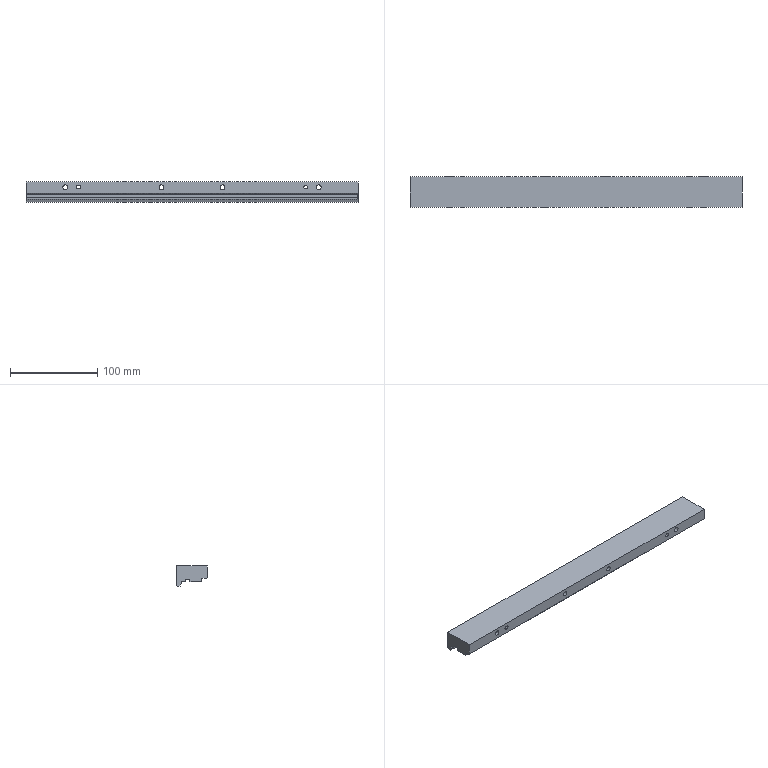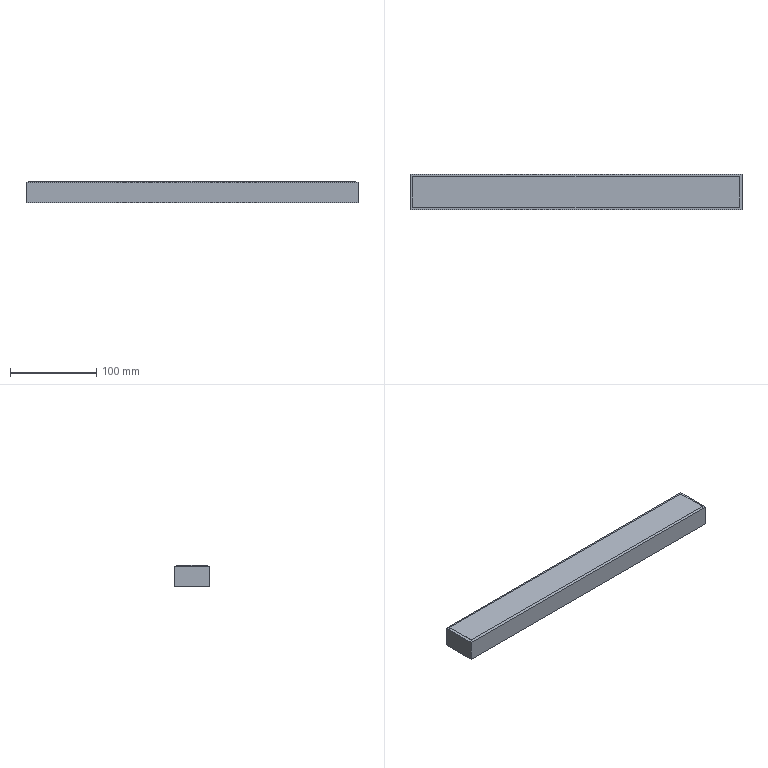CAM job | NX | 3-axis milling | part box 380 x 35 x 22.9 mm | stock box 386 x 41 x 24.9 mm
Tools:
number,name,description,diameter,corner_radius,flute_length,length,flutes
1,D50,Milling Tool-5 Parameters,50.0,0.0,50.0,75.0,2
3,D10,Milling Tool-5 Parameters,10.0,0.0,50.0,75.0,2
4,D10JING,Milling Tool-5 Parameters,10.0,0.0,50.0,75.0,2
2,D6A45,Milling Tool-5 Parameters,6.0,0.0,3.0,3.0,2
8,D6,Milling Tool-5 Parameters,6.0,0.0,50.0,75.0,2
10,D4,Milling Tool-5 Parameters,4.0,0.0,50.0,75.0,2
20,D6R0.5,Milling Tool-5 Parameters,6.0,0.5,50.0,75.0,2
Operations:
program,operation,operation_type,tool,method,geometry_group,spindle_rpm,surface_speed,feed_per_tooth,feed_cut,feed_plunge,cut_length_mm,path_length_mm,cut_time_min,machine_time_min
1-385-40-25毛胚,FLOOR_WALL,VolumeBased25DMillingOperation,D50,METHOD,A,6500.0,1286.0,0.0962,1250.0,100.0,448.0,502.0,0.3584,0.3638
1-385-40-25毛胚,ZLEVEL_PROFILE,ZLevelMilling,D10,METHOD,A,7000.0,219.0,0.2143,3000.0,1000.0,19933.435,20013.335,6.676,6.684
1-385-40-25毛胚,ZLEVEL_PROFILE_COPY_COPY_1_COPY_COPY_COPY_1,ZLevelMilling,D10JING,METHOD,A,7000.0,219.0,0.0714,1000.0,100.0,1729.097,1835.116,1.729,1.74
1-385-40-25毛胚,ZLEVEL_PROFILE_COPY_1_COPY_COPY_COPY_COPY_2_COPY,ZLevelMilling,D6A45,METHOD,A,7000.0,131.0,0.0714,1000.0,1000.0,839.121,901.121,0.8391,0.8453
2-385-40-25毛胚,FLOOR_WALL_COPY,VolumeBased25DMillingOperation,D50,METHOD,B,6500.0,1286.0,0.0962,1250.0,100.0,884.0,1426,0.7072,0.7614
2-385-40-25毛胚,FLOOR_WALL_1,VolumeBased25DMillingOperation,D10,METHOD,B,7000.0,219.0,0.2143,3000.0,1000.0,2750.061,2821.361,0.9207,0.9278
2-385-40-25毛胚,FLOOR_WALL_1_COPY,VolumeBased25DMillingOperation,D10,METHOD,B,7000.0,219.0,0.2143,3000.0,1000.0,9395.15,9458.85,3.136,3.142
2-385-40-25毛胚,FLOOR_WALL_1_COPY_1_1,VolumeBased25DMillingOperation,D6,METHOD,B,7000.0,87.0,0.0714,1000.0,100.0,5468.709,6463.497,5.469,5.594
2-385-40-25毛胚,FLOOR_WALL_1_1,VolumeBased25DMillingOperation,D4,METHOD,B,7000.0,87.0,0.1429,2000.0,1000.0,5415.9,5489.6,2.729,2.737
2-385-40-25毛胚,FLOOR_WALL_1_COPY_1,VolumeBased25DMillingOperation,D4,METHOD,B,7000.0,87.0,0.0714,1000.0,100.0,1561.599,1637.999,1.562,1.569
2-385-40-25毛胚,ZLEVEL_PROFILE_COPY_COPY_1_COPY_COPY_COPY_1_COPY_COPY,ZLevelMilling,D6R0.5,METHOD,B,7000.0,131.0,0.2143,3000.0,1000.0,14862.415,14926.006,4.955,4.961
2-385-40-25毛胚,ZLEVEL_PROFILE_COPY_1_COPY_COPY_COPY_COPY_2_COPY_COPY_COPY_COPY,ZLevelMilling,D6A45,METHOD,B,7000.0,131.0,0.0714,1000.0,1000.0,400.652,463.652,0.4007,0.407
2-385-40-25毛胚,ZLEVEL_PROFILE_COPY_1_COPY_COPY_COPY_COPY_2_COPY_COPY,ZLevelMilling,D6A45,METHOD,B,7000.0,131.0,0.0714,1000.0,1000.0,1188.735,1718.629,1.189,1.242
2-385-40-25毛胚,ZLEVEL_PROFILE_COPY_1_COPY_COPY_COPY_COPY_2_COPY_COPY_COPY,ZLevelMilling,D6A45,METHOD,B,7000.0,131.0,0.0714,1000.0,1000.0,396.744,478.344,0.3967,0.4049